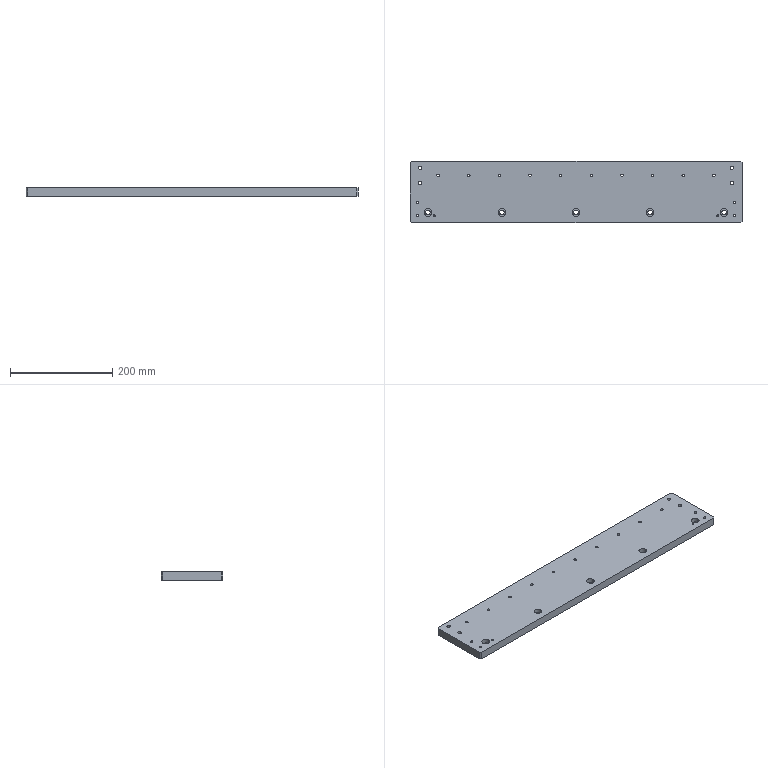Part | SolidWorks | features HoleWzd 5, Chamfer 1, Cut 1, Extrusion 1, ICE 1, MirrorPattern 1 | 1 solid | 75 faces | box 650 x 120 x 16 mm | volume 1230763 mm3 | cylinder 60 | plane 15 | commonest cylinder face diameters 5 x28 9 x10 15 x10 6.8 x8 3.3 x4